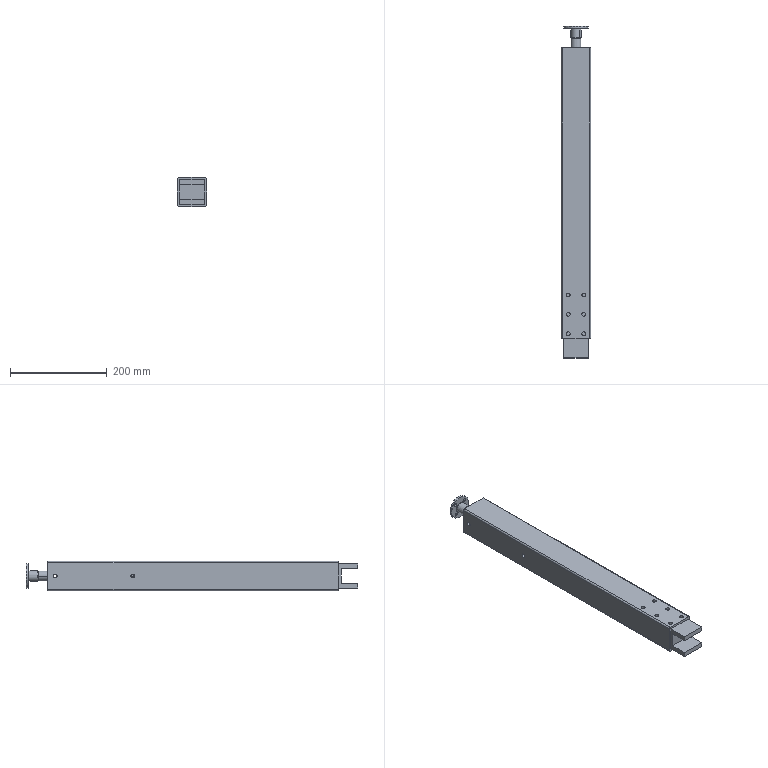Part | SolidWorks | 20 solids | 487 faces | box 60 x 685 x 60 mm | volume 1570398 mm3 | plane 244 | cylinder 194 | cone 40 | spline 5 | torus 4 | commonest cylinder face diameters 8 x62 32 x40 6 x24 5 x16 48 x14 20 x6